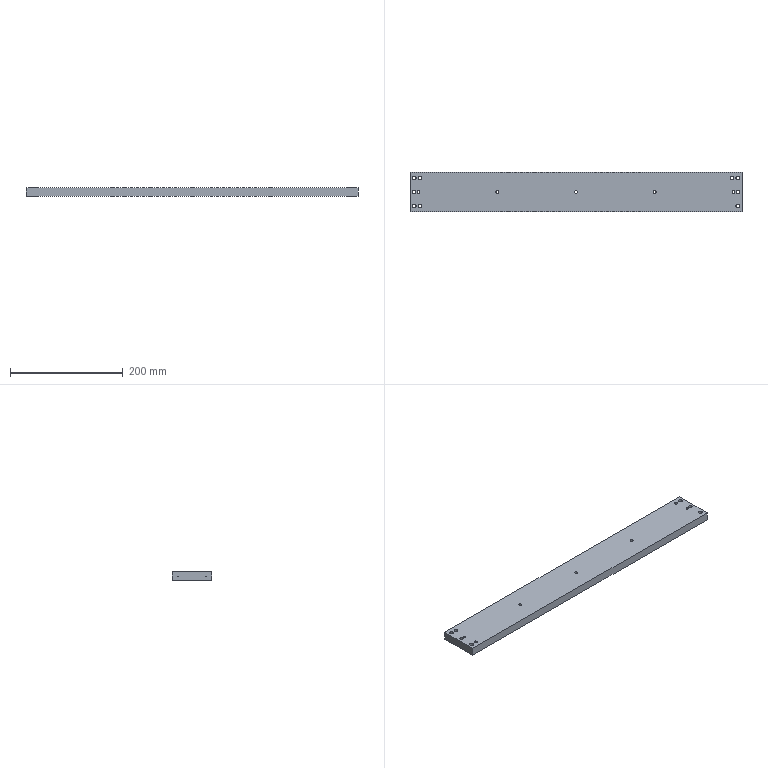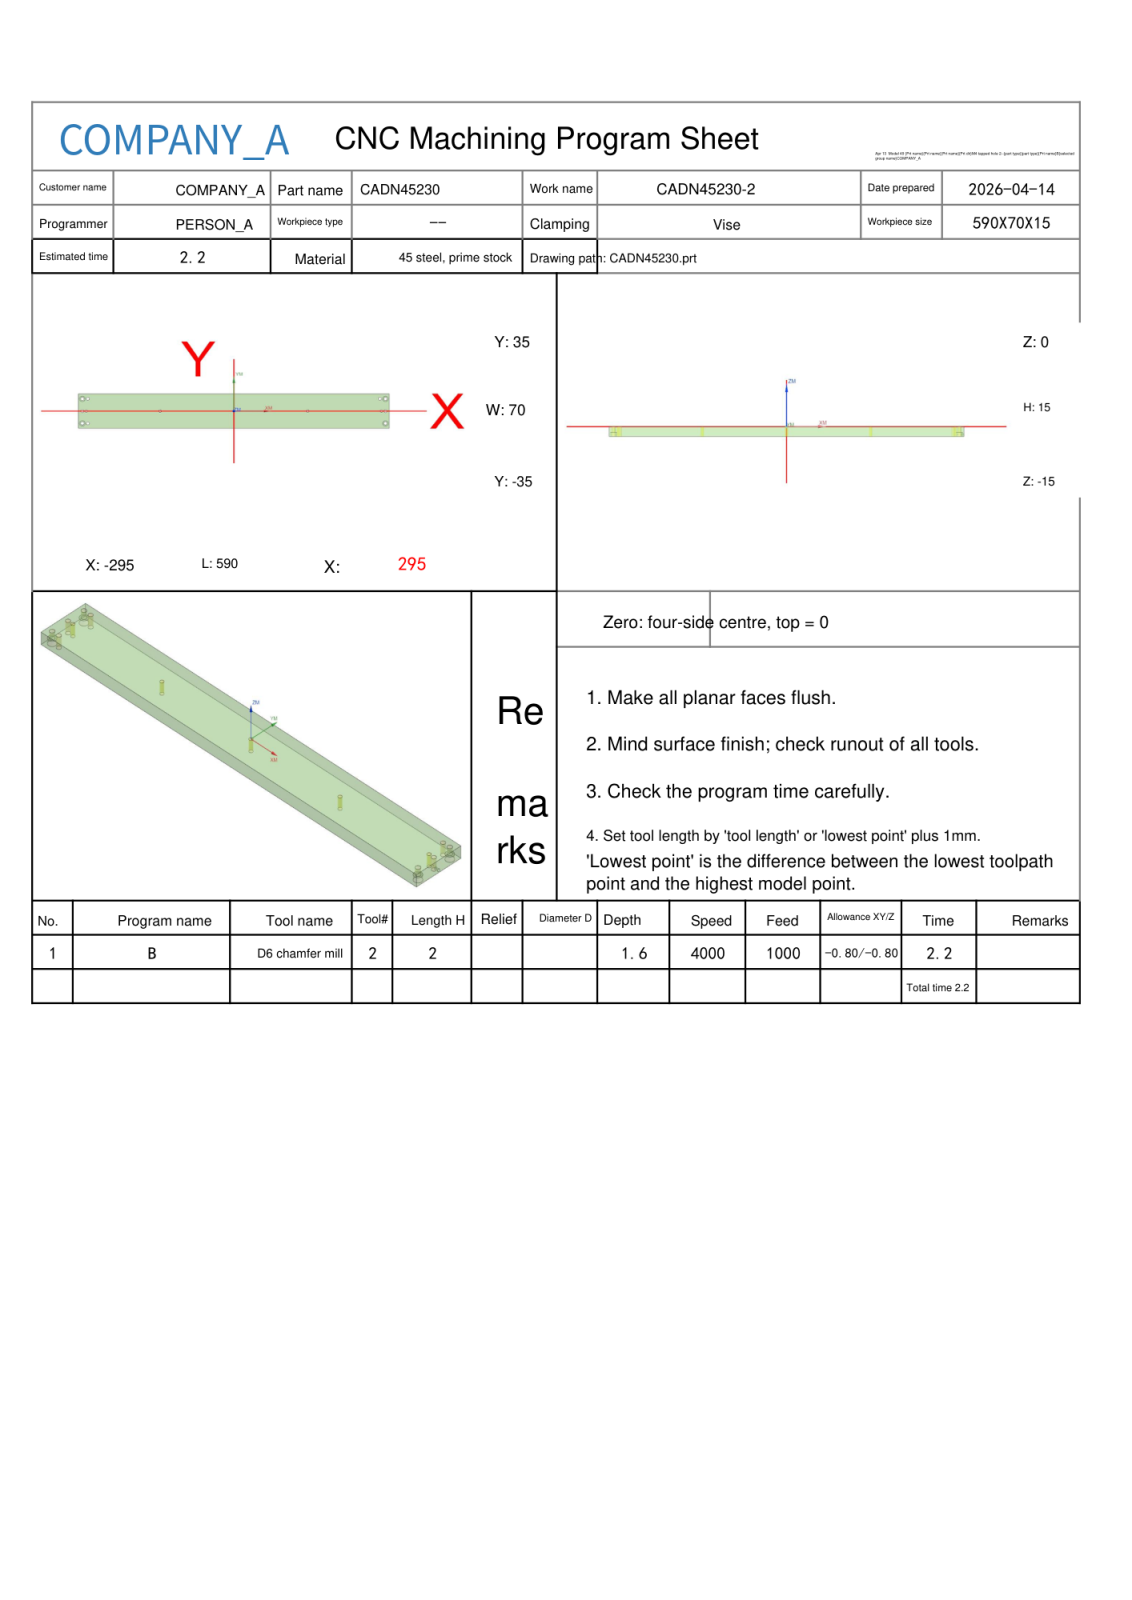NC program | NX | posted by the shop | part box 590 x 70 x 15 mm
Whole program:
%
O0001
(Machine time: 2.35 MIN)
(===Total Tool:1===)
(T2=D6 chamfer mill   D=6.   R=0.   D-  H02 Z=-1.6  )
G80 G90 G17 G49 G40
G91 G28 Z0
M01
N1 T02 M06
(D6 chamfer mill  D=6. R=0. H=02 ce=-0.80 di=-0.80)
G00 G90 G54 X-279.907 Y-.694 M03 S4000
G43 H02 Z20.
M08
Z-1.1
G01 Z-1.6 F300.
X-279.8 Y-1.5
G03 X-278.3 Y0.0 I0.0 J1.5
X-280. Y1.7 I-1.7 J0.0
X-281.7 Y0.0 I0.0 J-1.7
X-280. Y-1.7 I1.7 J0.0
X-278.3 Y0.0 I0.0 J1.7
X-279.8 Y1.5 I-1.5 J0.0
G01 X-279.907 Y.694
Z-1.1
G00 Z20.
X-139.907 Y-.694
Z-1.1
G01 Z-1.6
X-139.8 Y-1.5
G03 X-138.3 Y0.0 I0.0 J1.5
X-140. Y1.7 I-1.7 J0.0
X-141.7 Y0.0 I0.0 J-1.7
X-140. Y-1.7 I1.7 J0.0
X-138.3 Y0.0 I0.0 J1.7
X-139.8 Y1.5 I-1.5 J0.0
G01 X-139.907 Y.694
Z-1.1
G00 Z20.
X.093 Y-.694
Z-1.1
G01 Z-1.6
X.2 Y-1.5
G03 X1.7 Y0.0 I0.0 J1.5
X0.0 Y1.7 I-1.7 J0.0
X-1.7 Y0.0 I0.0 J-1.7
X0.0 Y-1.7 I1.7 J0.0
X1.7 Y0.0 I0.0 J1.7
X.2 Y1.5 I-1.5 J0.0
G01 X.093 Y.694
Z-1.1
G00 Z20.
X140.093 Y-.694
Z-1.1
G01 Z-1.6
X140.2 Y-1.5
G03 X141.7 Y0.0 I0.0 J1.5
X140. Y1.7 I-1.7 J0.0
X138.3 Y0.0 I0.0 J-1.7
X140. Y-1.7 I1.7 J0.0
X141.7 Y0.0 I0.0 J1.7
X140.2 Y1.5 I-1.5 J0.0
G01 X140.093 Y.694
Z-1.1
G00 Z20.
X280.093 Y-.694
Z-1.1
G01 Z-1.6
X280.2 Y-1.5
G03 X281.7 Y0.0 I0.0 J1.5
X280. Y1.7 I-1.7 J0.0
X278.3 Y0.0 I0.0 J-1.7
X280. Y-1.7 I1.7 J0.0
X281.7 Y0.0 I0.0 J1.7
X280.2 Y1.5 I-1.5 J0.0
G01 X280.093 Y.694
Z-1.1
G00 Z20.
G00 G90 X287.593 Y-.694 M03 S4000
Z20.
Z-1.1
G01 Z-1.6 F600.
X287.7 Y-1.5
G03 X289.2 Y0.0 I0.0 J1.5
X287.5 Y1.7 I-1.7 J0.0
X285.8 Y0.0 I0.0 J-1.7
X287.5 Y-1.7 I1.7 J0.0
X289.2 Y0.0 I0.0 J1.7
X287.7 Y1.5 I-1.5 J0.0
G01 X287.593 Y.694
Z-1.1
G00 Z20.
X277.093 Y24.306
Z-1.1
G01 Z-1.6
X277.2 Y23.5
G03 X278.7 Y25. I0.0 J1.5
X277. Y26.7 I-1.7 J0.0
X275.3 Y25. I0.0 J-1.7
X277. Y23.3 I1.7 J0.0
X278.7 Y25. I0.0 J1.7
X277.2 Y26.5 I-1.5 J0.0
G01 X277.093 Y25.694
Z-1.1
G00 Z20.
X-276.907 Y24.306
Z-1.1
G01 Z-1.6
X-276.8 Y23.5
G03 X-275.3 Y25. I0.0 J1.5
X-277. Y26.7 I-1.7 J0.0
X-278.7 Y25. I0.0 J-1.7
X-277. Y23.3 I1.7 J0.0
X-275.3 Y25. I0.0 J1.7
X-276.8 Y26.5 I-1.5 J0.0
G01 X-276.907 Y25.694
Z-1.1
G00 Z20.
X-287.407 Y-.694
Z-1.1
G01 Z-1.6
X-287.3 Y-1.5
G03 X-285.8 Y0.0 I0.0 J1.5
X-287.5 Y1.7 I-1.7 J0.0
X-289.2 Y0.0 I0.0 J-1.7
X-287.5 Y-1.7 I1.7 J0.0
X-285.8 Y0.0 I0.0 J1.7
X-287.3 Y1.5 I-1.5 J0.0
G01 X-287.407 Y.694
Z-1.1
G00 Z20.
X-276.907 Y-25.694
Z-1.1
G01 Z-1.6
X-276.8 Y-26.5
G03 X-275.3 Y-25. I0.0 J1.5
X-277. Y-23.3 I-1.7 J0.0
X-278.7 Y-25. I0.0 J-1.7
X-277. Y-26.7 I1.7 J0.0
X-275.3 Y-25. I0.0 J1.7
X-276.8 Y-23.5 I-1.5 J0.0
G01 X-276.907 Y-24.306
Z-1.1
G00 Z20.
G00 G90 X-287.184 Y24.051 M03 S4000
Z20.
Z-1.1
G01 Z-1.6 F600.
X-287. Y23.5
G03 X-285.5 Y25. I0.0 J1.5
X-287.5 Y27. I-2. J0.0
X-289.5 Y25. I0.0 J-2.
X-287.5 Y23. I2. J0.0
X-285.5 Y25. I0.0 J2.
X-287. Y26.5 I-1.5 J0.0
G01 X-287.184 Y25.949
Z-1.1
G00 Z20.
Y-25.949
Z-1.1
G01 Z-1.6
X-287. Y-26.5
G03 X-285.5 Y-25. I0.0 J1.5
X-287.5 Y-23. I-2. J0.0
X-289.5 Y-25. I0.0 J-2.
X-287.5 Y-27. I2. J0.0
X-285.5 Y-25. I0.0 J2.
X-287. Y-23.5 I-1.5 J0.0
G01 X-287.184 Y-24.051
Z-1.1
G00 Z20.
X287.816 Y-25.949
Z-1.1
G01 Z-1.6
X288. Y-26.5
G03 X289.5 Y-25. I0.0 J1.5
X287.5 Y-23. I-2. J0.0
X285.5 Y-25. I0.0 J-2.
X287.5 Y-27. I2. J0.0
X289.5 Y-25. I0.0 J2.
X288. Y-23.5 I-1.5 J0.0
G01 X287.816 Y-24.051
Z-1.1
G00 Z20.
Y24.051
Z-1.1
G01 Z-1.6
X288. Y23.5
G03 X289.5 Y25. I0.0 J1.5
X287.5 Y27. I-2. J0.0
X285.5 Y25. I0.0 J-2.
X287.5 Y23. I2. J0.0
X289.5 Y25. I0.0 J2.
X288. Y26.5 I-1.5 J0.0
G01 X287.816 Y25.949
Z-1.1
G00 Z20.
G00 G90 X-295.9 Y26.422 M03 S4000
Z20.
Z2.5
G01 Y34.7 Z-.513 F1000.
Y34.785 Z-.544
X-295.866 Y34.997 Z-.622
X-295.794 Y35.199 Z-.7
X-295.688 Y35.386 Z-.778
X-295.551 Y35.551 Z-.857
X-295.386 Y35.688 Z-.935
X-295.199 Y35.794 Z-1.013
X-294.997 Y35.866 Z-1.091
X-294.785 Y35.9 Z-1.169
X-294.7 Z-1.2
X294.7
G02 X295.9 Y34.7 I0.0 J-1.2
G01 Y-34.7
G02 X294.7 Y-35.9 I-1.2 J0.0
G01 X-294.7
G02 X-295.9 Y-34.7 I0.0 J1.2
G01 Y34.7
G02 X-294.7 Y35.9 I1.2 J0.0
G01 X-294.2
Z1.3
G00 Z20.
M05
M09
G91 G28 Z0.0
G91 G28 Y0.0
M30
%